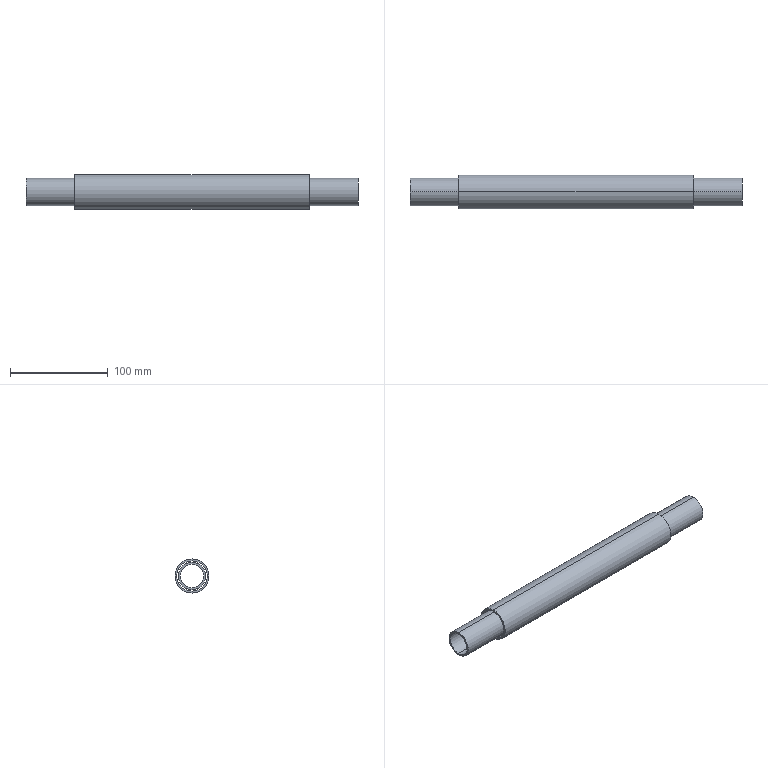Part | STEP file | VIB-C1-1-8-vibration damping pipe 28_default_machined_ | 2 solids | 12 faces | box 340 x 35 x 35 mm | volume 105306 mm3 | cylinder 8 | plane 4 | commonest cylinder face diameters 24 x2 28 x2 31 x2 35 x2
STEP:
#1=CARTESIAN_POINT('',(0.,0.,0.));
#2=DIRECTION('',(0.,0.,1.));
#3=DIRECTION('',(1.,0.,0.));
#4=AXIS2_PLACEMENT_3D('',#1,#2,#3);
#5=CARTESIAN_POINT('',(340.,0.,14.));
#6=VERTEX_POINT('',#5);
#7=CARTESIAN_POINT('',(340.,0.,-14.));
#8=VERTEX_POINT('',#7);
#9=CARTESIAN_POINT('',(340.,0.,0.));
#10=DIRECTION('',(-1.,0.,0.));
#11=DIRECTION('',(0.,0.,1.));
#12=AXIS2_PLACEMENT_3D('',#9,#10,#11);
#13=CIRCLE('',#12,14.);
#14=CARTESIAN_POINT('',(340.,0.,0.));
#15=DIRECTION('',(-1.,0.,0.));
#16=DIRECTION('',(0.,0.,1.));
#17=AXIS2_PLACEMENT_3D('',#14,#15,#16);
#18=CYLINDRICAL_SURFACE('',#17,14.);
#19=CARTESIAN_POINT('',(0.,0.));
#20=DIRECTION('',(1.,0.));
#21=VECTOR('',#20,1.);
#22=LINE('',#19,#21);
#23=(GEOMETRIC_REPRESENTATION_CONTEXT(2)PARAMETRIC_REPRESENTATION_CONTEXT()REPRESENTATION_CONTEXT('',''));
#24=DEFINITIONAL_REPRESENTATION('',(#22),#23);
#25=PCURVE('',#18,#24);
#26=CARTESIAN_POINT('',(340.,0.,0.));
#27=DIRECTION('',(1.,0.,0.));
#28=DIRECTION('',(0.,0.,-1.));
#29=AXIS2_PLACEMENT_3D('',#26,#27,#28);
#30=PLANE('',#29);
#31=CARTESIAN_POINT('',(-14.,0.));
#32=CARTESIAN_POINT('',(-14.,24.249));
#33=CARTESIAN_POINT('',(7.,12.124));
#34=CARTESIAN_POINT('',(28.,0.));
#35=CARTESIAN_POINT('',(7.,-12.124));
#36=CARTESIAN_POINT('',(-14.,-24.249));
#37=CARTESIAN_POINT('',(-14.,0.));
#38=(BOUNDED_CURVE()B_SPLINE_CURVE(2,(#31,#32,#33,#34,#35,#36,#37),.UNSPECIFIED.,.T.,.F.)B_SPLINE_CURVE_WITH_KNOTS((1,2,2,2,2,1),(-2.094,0.,2.094,4.189,6.283,8.378),.UNSPECIFIED.)CURVE()GEOMETRIC_REPRESENTATION_ITEM()RATIONAL_B_SPLINE_CURVE((1.,0.5,1.,0.5,1.,0.5,1.))REPRESENTATION_ITEM(''));
#39=(GEOMETRIC_REPRESENTATION_CONTEXT(2)PARAMETRIC_REPRESENTATION_CONTEXT()REPRESENTATION_CONTEXT('',''));
#40=DEFINITIONAL_REPRESENTATION('',(#38),#39);
#41=PCURVE('',#30,#40);
#42=SURFACE_CURVE('',#13,(#25,#41),.PCURVE_S1.);
#43=EDGE_CURVE('',#6,#8,#42,.T.);
#44=ORIENTED_EDGE('',*,*,#43,.T.);
#45=CARTESIAN_POINT('',(0.,0.,-14.));
#46=VERTEX_POINT('',#45);
#47=CARTESIAN_POINT('',(340.,0.,-14.));
#48=DIRECTION('',(-1.,0.,0.));
#49=VECTOR('',#48,1.);
#50=LINE('',#47,#49);
#51=CARTESIAN_POINT('',(3.142,0.));
#52=DIRECTION('',(0.,1.));
#53=VECTOR('',#52,1.);
#54=LINE('',#51,#53);
#55=(GEOMETRIC_REPRESENTATION_CONTEXT(2)PARAMETRIC_REPRESENTATION_CONTEXT()REPRESENTATION_CONTEXT('',''));
#56=DEFINITIONAL_REPRESENTATION('',(#54),#55);
#57=PCURVE('',#18,#56);
#58=CARTESIAN_POINT('',(340.,0.,0.));
#59=DIRECTION('',(-1.,0.,0.));
#60=DIRECTION('',(0.,0.,1.));
#61=AXIS2_PLACEMENT_3D('',#58,#59,#60);
#62=CYLINDRICAL_SURFACE('',#61,14.);
#63=CARTESIAN_POINT('',(3.142,0.));
#64=DIRECTION('',(0.,1.));
#65=VECTOR('',#64,1.);
#66=LINE('',#63,#65);
#67=(GEOMETRIC_REPRESENTATION_CONTEXT(2)PARAMETRIC_REPRESENTATION_CONTEXT()REPRESENTATION_CONTEXT('',''));
#68=DEFINITIONAL_REPRESENTATION('',(#66),#67);
#69=PCURVE('',#62,#68);
#70=SURFACE_CURVE('',#50,(#57,#69),.PCURVE_S1.);
#71=EDGE_CURVE('',#8,#46,#70,.T.);
#72=ORIENTED_EDGE('',*,*,#71,.T.);
#73=CARTESIAN_POINT('',(0.,0.,14.));
#74=VERTEX_POINT('',#73);
#75=CARTESIAN_POINT('',(0.,0.,0.));
#76=DIRECTION('',(1.,0.,0.));
#77=DIRECTION('',(0.,0.,1.));
#78=AXIS2_PLACEMENT_3D('',#75,#76,#77);
#79=CIRCLE('',#78,14.);
#80=CARTESIAN_POINT('',(6.283,340.));
#81=DIRECTION('',(-1.,0.));
#82=VECTOR('',#81,1.);
#83=LINE('',#80,#82);
#84=(GEOMETRIC_REPRESENTATION_CONTEXT(2)PARAMETRIC_REPRESENTATION_CONTEXT()REPRESENTATION_CONTEXT('',''));
#85=DEFINITIONAL_REPRESENTATION('',(#83),#84);
#86=PCURVE('',#18,#85);
#87=CARTESIAN_POINT('',(0.,0.,0.));
#88=DIRECTION('',(1.,0.,0.));
#89=DIRECTION('',(0.,0.,-1.));
#90=AXIS2_PLACEMENT_3D('',#87,#88,#89);
#91=PLANE('',#90);
#92=CARTESIAN_POINT('',(0.,0.));
#93=DIRECTION('',(-1.,0.));
#94=AXIS2_PLACEMENT_2D('',#92,#93);
#95=CIRCLE('',#94,14.);
#96=(GEOMETRIC_REPRESENTATION_CONTEXT(2)PARAMETRIC_REPRESENTATION_CONTEXT()REPRESENTATION_CONTEXT('',''));
#97=DEFINITIONAL_REPRESENTATION('',(#95),#96);
#98=PCURVE('',#91,#97);
#99=SURFACE_CURVE('',#79,(#86,#98),.PCURVE_S1.);
#100=EDGE_CURVE('',#46,#74,#99,.T.);
#101=ORIENTED_EDGE('',*,*,#100,.T.);
#102=CARTESIAN_POINT('',(340.,0.,14.));
#103=DIRECTION('',(-1.,0.,0.));
#104=VECTOR('',#103,1.);
#105=LINE('',#102,#104);
#106=CARTESIAN_POINT('',(0.,0.));
#107=DIRECTION('',(0.,1.));
#108=VECTOR('',#107,1.);
#109=LINE('',#106,#108);
#110=(GEOMETRIC_REPRESENTATION_CONTEXT(2)PARAMETRIC_REPRESENTATION_CONTEXT()REPRESENTATION_CONTEXT('',''));
#111=DEFINITIONAL_REPRESENTATION('',(#109),#110);
#112=PCURVE('',#18,#111);
#113=CARTESIAN_POINT('',(6.283,0.));
#114=DIRECTION('',(0.,1.));
#115=VECTOR('',#114,1.);
#116=LINE('',#113,#115);
#117=(GEOMETRIC_REPRESENTATION_CONTEXT(2)PARAMETRIC_REPRESENTATION_CONTEXT()REPRESENTATION_CONTEXT('',''));
#118=DEFINITIONAL_REPRESENTATION('',(#116),#117);
#119=PCURVE('',#62,#118);
#120=SURFACE_CURVE('',#105,(#112,#119),.PCURVE_S1.);
#121=EDGE_CURVE('',#6,#74,#120,.T.);
#122=ORIENTED_EDGE('',*,*,#121,.F.);
#123=EDGE_LOOP('',(#44,#72,#101,#122));
#124=FACE_BOUND('',#123,.T.);
#125=ADVANCED_FACE('',(#124),#18,.T.);
#126=CARTESIAN_POINT('',(340.,0.,12.));
#127=VERTEX_POINT('',#126);
#128=CARTESIAN_POINT('',(0.,0.,12.));
#129=VERTEX_POINT('',#128);
#130=CARTESIAN_POINT('',(340.,0.,12.));
#131=DIRECTION('',(-1.,0.,0.));
#132=VECTOR('',#131,1.);
#133=LINE('',#130,#132);
#134=CARTESIAN_POINT('',(340.,0.,0.));
#135=DIRECTION('',(-1.,0.,0.));
#136=DIRECTION('',(0.,0.,1.));
#137=AXIS2_PLACEMENT_3D('',#134,#135,#136);
#138=CYLINDRICAL_SURFACE('',#137,12.);
#139=CARTESIAN_POINT('',(6.283,0.));
#140=DIRECTION('',(0.,1.));
#141=VECTOR('',#140,1.);
#142=LINE('',#139,#141);
#143=(GEOMETRIC_REPRESENTATION_CONTEXT(2)PARAMETRIC_REPRESENTATION_CONTEXT()REPRESENTATION_CONTEXT('',''));
#144=DEFINITIONAL_REPRESENTATION('',(#142),#143);
#145=PCURVE('',#138,#144);
#146=CARTESIAN_POINT('',(340.,0.,0.));
#147=DIRECTION('',(-1.,0.,0.));
#148=DIRECTION('',(0.,0.,1.));
#149=AXIS2_PLACEMENT_3D('',#146,#147,#148);
#150=CYLINDRICAL_SURFACE('',#149,12.);
#151=CARTESIAN_POINT('',(0.,0.));
#152=DIRECTION('',(0.,1.));
#153=VECTOR('',#152,1.);
#154=LINE('',#151,#153);
#155=(GEOMETRIC_REPRESENTATION_CONTEXT(2)PARAMETRIC_REPRESENTATION_CONTEXT()REPRESENTATION_CONTEXT('',''));
#156=DEFINITIONAL_REPRESENTATION('',(#154),#155);
#157=PCURVE('',#150,#156);
#158=SURFACE_CURVE('',#133,(#145,#157),.PCURVE_S1.);
#159=EDGE_CURVE('',#127,#129,#158,.T.);
#160=ORIENTED_EDGE('',*,*,#159,.T.);
#161=CARTESIAN_POINT('',(0.,0.,-12.));
#162=VERTEX_POINT('',#161);
#163=CARTESIAN_POINT('',(0.,0.,0.));
#164=DIRECTION('',(-1.,0.,0.));
#165=DIRECTION('',(0.,0.,1.));
#166=AXIS2_PLACEMENT_3D('',#163,#164,#165);
#167=CIRCLE('',#166,12.);
#168=CARTESIAN_POINT('',(0.,340.));
#169=DIRECTION('',(1.,0.));
#170=VECTOR('',#169,1.);
#171=LINE('',#168,#170);
#172=(GEOMETRIC_REPRESENTATION_CONTEXT(2)PARAMETRIC_REPRESENTATION_CONTEXT()REPRESENTATION_CONTEXT('',''));
#173=DEFINITIONAL_REPRESENTATION('',(#171),#172);
#174=PCURVE('',#138,#173);
#175=CARTESIAN_POINT('',(-12.,0.));
#176=CARTESIAN_POINT('',(-12.,20.785));
#177=CARTESIAN_POINT('',(6.,10.392));
#178=CARTESIAN_POINT('',(24.,0.));
#179=CARTESIAN_POINT('',(6.,-10.392));
#180=CARTESIAN_POINT('',(-12.,-20.785));
#181=CARTESIAN_POINT('',(-12.,0.));
#182=(BOUNDED_CURVE()B_SPLINE_CURVE(2,(#175,#176,#177,#178,#179,#180,#181),.UNSPECIFIED.,.T.,.F.)B_SPLINE_CURVE_WITH_KNOTS((1,2,2,2,2,1),(-2.094,0.,2.094,4.189,6.283,8.378),.UNSPECIFIED.)CURVE()GEOMETRIC_REPRESENTATION_ITEM()RATIONAL_B_SPLINE_CURVE((1.,0.5,1.,0.5,1.,0.5,1.))REPRESENTATION_ITEM(''));
#183=(GEOMETRIC_REPRESENTATION_CONTEXT(2)PARAMETRIC_REPRESENTATION_CONTEXT()REPRESENTATION_CONTEXT('',''));
#184=DEFINITIONAL_REPRESENTATION('',(#182),#183);
#185=PCURVE('',#91,#184);
#186=SURFACE_CURVE('',#167,(#174,#185),.PCURVE_S1.);
#187=EDGE_CURVE('',#162,#129,#186,.T.);
#188=ORIENTED_EDGE('',*,*,#187,.F.);
#189=CARTESIAN_POINT('',(340.,0.,-12.));
#190=VERTEX_POINT('',#189);
#191=CARTESIAN_POINT('',(340.,0.,-12.));
#192=DIRECTION('',(-1.,0.,0.));
#193=VECTOR('',#192,1.);
#194=LINE('',#191,#193);
#195=CARTESIAN_POINT('',(3.142,0.));
#196=DIRECTION('',(0.,1.));
#197=VECTOR('',#196,1.);
#198=LINE('',#195,#197);
#199=(GEOMETRIC_REPRESENTATION_CONTEXT(2)PARAMETRIC_REPRESENTATION_CONTEXT()REPRESENTATION_CONTEXT('',''));
#200=DEFINITIONAL_REPRESENTATION('',(#198),#199);
#201=PCURVE('',#138,#200);
#202=CARTESIAN_POINT('',(3.142,0.));
#203=DIRECTION('',(0.,1.));
#204=VECTOR('',#203,1.);
#205=LINE('',#202,#204);
#206=(GEOMETRIC_REPRESENTATION_CONTEXT(2)PARAMETRIC_REPRESENTATION_CONTEXT()REPRESENTATION_CONTEXT('',''));
#207=DEFINITIONAL_REPRESENTATION('',(#205),#206);
#208=PCURVE('',#150,#207);
#209=SURFACE_CURVE('',#194,(#201,#208),.PCURVE_S1.);
#210=EDGE_CURVE('',#190,#162,#209,.T.);
#211=ORIENTED_EDGE('',*,*,#210,.F.);
#212=CARTESIAN_POINT('',(340.,0.,0.));
#213=DIRECTION('',(-1.,0.,0.));
#214=DIRECTION('',(0.,0.,1.));
#215=AXIS2_PLACEMENT_3D('',#212,#213,#214);
#216=CIRCLE('',#215,12.);
#217=CARTESIAN_POINT('',(0.,0.));
#218=DIRECTION('',(1.,0.));
#219=VECTOR('',#218,1.);
#220=LINE('',#217,#219);
#221=(GEOMETRIC_REPRESENTATION_CONTEXT(2)PARAMETRIC_REPRESENTATION_CONTEXT()REPRESENTATION_CONTEXT('',''));
#222=DEFINITIONAL_REPRESENTATION('',(#220),#221);
#223=PCURVE('',#138,#222);
#224=CARTESIAN_POINT('',(-12.,0.));
#225=CARTESIAN_POINT('',(-12.,20.785));
#226=CARTESIAN_POINT('',(6.,10.392));
#227=CARTESIAN_POINT('',(24.,0.));
#228=CARTESIAN_POINT('',(6.,-10.392));
#229=CARTESIAN_POINT('',(-12.,-20.785));
#230=CARTESIAN_POINT('',(-12.,0.));
#231=(BOUNDED_CURVE()B_SPLINE_CURVE(2,(#224,#225,#226,#227,#228,#229,#230),.UNSPECIFIED.,.T.,.F.)B_SPLINE_CURVE_WITH_KNOTS((1,2,2,2,2,1),(-2.094,0.,2.094,4.189,6.283,8.378),.UNSPECIFIED.)CURVE()GEOMETRIC_REPRESENTATION_ITEM()RATIONAL_B_SPLINE_CURVE((1.,0.5,1.,0.5,1.,0.5,1.))REPRESENTATION_ITEM(''));
#232=(GEOMETRIC_REPRESENTATION_CONTEXT(2)PARAMETRIC_REPRESENTATION_CONTEXT()REPRESENTATION_CONTEXT('',''));
#233=DEFINITIONAL_REPRESENTATION('',(#231),#232);
#234=PCURVE('',#30,#233);
#235=SURFACE_CURVE('',#216,(#223,#234),.PCURVE_S1.);
#236=EDGE_CURVE('',#190,#127,#235,.T.);
#237=ORIENTED_EDGE('',*,*,#236,.T.);
#238=EDGE_LOOP('',(#160,#188,#211,#237));
#239=FACE_BOUND('',#238,.F.);
#240=ADVANCED_FACE('',(#239),#138,.F.);
#241=ORIENTED_EDGE('',*,*,#71,.F.);
#242=CARTESIAN_POINT('',(340.,0.,0.));
#243=DIRECTION('',(-1.,0.,0.));
#244=DIRECTION('',(0.,0.,1.));
#245=AXIS2_PLACEMENT_3D('',#242,#243,#244);
#246=CIRCLE('',#245,14.);
#247=CARTESIAN_POINT('',(0.,0.));
#248=DIRECTION('',(1.,0.));
#249=VECTOR('',#248,1.);
#250=LINE('',#247,#249);
#251=(GEOMETRIC_REPRESENTATION_CONTEXT(2)PARAMETRIC_REPRESENTATION_CONTEXT()REPRESENTATION_CONTEXT('',''));
#252=DEFINITIONAL_REPRESENTATION('',(#250),#251);
#253=PCURVE('',#62,#252);
#254=CARTESIAN_POINT('',(-14.,0.));
#255=CARTESIAN_POINT('',(-14.,24.249));
#256=CARTESIAN_POINT('',(7.,12.124));
#257=CARTESIAN_POINT('',(28.,0.));
#258=CARTESIAN_POINT('',(7.,-12.124));
#259=CARTESIAN_POINT('',(-14.,-24.249));
#260=CARTESIAN_POINT('',(-14.,0.));
#261=(BOUNDED_CURVE()B_SPLINE_CURVE(2,(#254,#255,#256,#257,#258,#259,#260),.UNSPECIFIED.,.T.,.F.)B_SPLINE_CURVE_WITH_KNOTS((1,2,2,2,2,1),(-2.094,0.,2.094,4.189,6.283,8.378),.UNSPECIFIED.)CURVE()GEOMETRIC_REPRESENTATION_ITEM()RATIONAL_B_SPLINE_CURVE((1.,0.5,1.,0.5,1.,0.5,1.))REPRESENTATION_ITEM(''));
#262=(GEOMETRIC_REPRESENTATION_CONTEXT(2)PARAMETRIC_REPRESENTATION_CONTEXT()REPRESENTATION_CONTEXT('',''));
#263=DEFINITIONAL_REPRESENTATION('',(#261),#262);
#264=PCURVE('',#30,#263);
#265=SURFACE_CURVE('',#246,(#253,#264),.PCURVE_S1.);
#266=EDGE_CURVE('',#8,#6,#265,.T.);
#267=ORIENTED_EDGE('',*,*,#266,.T.);
#268=ORIENTED_EDGE('',*,*,#121,.T.);
#269=CARTESIAN_POINT('',(0.,0.,0.));
#270=DIRECTION('',(1.,0.,0.));
#271=DIRECTION('',(0.,0.,1.));
#272=AXIS2_PLACEMENT_3D('',#269,#270,#271);
#273=CIRCLE('',#272,14.);
#274=CARTESIAN_POINT('',(6.283,340.));
#275=DIRECTION('',(-1.,0.));
#276=VECTOR('',#275,1.);
#277=LINE('',#274,#276);
#278=(GEOMETRIC_REPRESENTATION_CONTEXT(2)PARAMETRIC_REPRESENTATION_CONTEXT()REPRESENTATION_CONTEXT('',''));
#279=DEFINITIONAL_REPRESENTATION('',(#277),#278);
#280=PCURVE('',#62,#279);
#281=CARTESIAN_POINT('',(0.,0.));
#282=DIRECTION('',(-1.,0.));
#283=AXIS2_PLACEMENT_2D('',#281,#282);
#284=CIRCLE('',#283,14.);
#285=(GEOMETRIC_REPRESENTATION_CONTEXT(2)PARAMETRIC_REPRESENTATION_CONTEXT()REPRESENTATION_CONTEXT('',''));
#286=DEFINITIONAL_REPRESENTATION('',(#284),#285);
#287=PCURVE('',#91,#286);
#288=SURFACE_CURVE('',#273,(#280,#287),.PCURVE_S1.);
#289=EDGE_CURVE('',#74,#46,#288,.T.);
#290=ORIENTED_EDGE('',*,*,#289,.T.);
#291=EDGE_LOOP('',(#241,#267,#268,#290));
#292=FACE_BOUND('',#291,.T.);
#293=ADVANCED_FACE('',(#292),#62,.T.);
#294=ORIENTED_EDGE('',*,*,#289,.F.);
#295=ORIENTED_EDGE('',*,*,#100,.F.);
#296=EDGE_LOOP('',(#294,#295));
#297=FACE_BOUND('',#296,.T.);
#298=CARTESIAN_POINT('',(0.,0.,0.));
#299=DIRECTION('',(-1.,0.,0.));
#300=DIRECTION('',(0.,0.,1.));
#301=AXIS2_PLACEMENT_3D('',#298,#299,#300);
#302=CIRCLE('',#301,12.);
#303=CARTESIAN_POINT('',(-12.,0.));
#304=CARTESIAN_POINT('',(-12.,20.785));
#305=CARTESIAN_POINT('',(6.,10.392));
#306=CARTESIAN_POINT('',(24.,0.));
#307=CARTESIAN_POINT('',(6.,-10.392));
#308=CARTESIAN_POINT('',(-12.,-20.785));
#309=CARTESIAN_POINT('',(-12.,0.));
#310=(BOUNDED_CURVE()B_SPLINE_CURVE(2,(#303,#304,#305,#306,#307,#308,#309),.UNSPECIFIED.,.T.,.F.)B_SPLINE_CURVE_WITH_KNOTS((1,2,2,2,2,1),(-2.094,0.,2.094,4.189,6.283,8.378),.UNSPECIFIED.)CURVE()GEOMETRIC_REPRESENTATION_ITEM()RATIONAL_B_SPLINE_CURVE((1.,0.5,1.,0.5,1.,0.5,1.))REPRESENTATION_ITEM(''));
#311=(GEOMETRIC_REPRESENTATION_CONTEXT(2)PARAMETRIC_REPRESENTATION_CONTEXT()REPRESENTATION_CONTEXT('',''));
#312=DEFINITIONAL_REPRESENTATION('',(#310),#311);
#313=PCURVE('',#91,#312);
#314=CARTESIAN_POINT('',(0.,340.));
#315=DIRECTION('',(1.,0.));
#316=VECTOR('',#315,1.);
#317=LINE('',#314,#316);
#318=(GEOMETRIC_REPRESENTATION_CONTEXT(2)PARAMETRIC_REPRESENTATION_CONTEXT()REPRESENTATION_CONTEXT('',''));
#319=DEFINITIONAL_REPRESENTATION('',(#317),#318);
#320=PCURVE('',#150,#319);
#321=SURFACE_CURVE('',#302,(#313,#320),.PCURVE_S1.);
#322=EDGE_CURVE('',#129,#162,#321,.T.);
#323=ORIENTED_EDGE('',*,*,#322,.F.);
#324=ORIENTED_EDGE('',*,*,#187,.F.);
#325=EDGE_LOOP('',(#323,#324));
#326=FACE_BOUND('',#325,.T.);
#327=ADVANCED_FACE('',(#297,#326),#91,.F.);
#328=ORIENTED_EDGE('',*,*,#43,.F.);
#329=ORIENTED_EDGE('',*,*,#266,.F.);
#330=EDGE_LOOP('',(#328,#329));
#331=FACE_BOUND('',#330,.T.);
#332=CARTESIAN_POINT('',(340.,0.,0.));
#333=DIRECTION('',(-1.,0.,0.));
#334=DIRECTION('',(0.,0.,1.));
#335=AXIS2_PLACEMENT_3D('',#332,#333,#334);
#336=CIRCLE('',#335,12.);
#337=CARTESIAN_POINT('',(-12.,0.));
#338=CARTESIAN_POINT('',(-12.,20.785));
#339=CARTESIAN_POINT('',(6.,10.392));
#340=CARTESIAN_POINT('',(24.,0.));
#341=CARTESIAN_POINT('',(6.,-10.392));
#342=CARTESIAN_POINT('',(-12.,-20.785));
#343=CARTESIAN_POINT('',(-12.,0.));
#344=(BOUNDED_CURVE()B_SPLINE_CURVE(2,(#337,#338,#339,#340,#341,#342,#343),.UNSPECIFIED.,.T.,.F.)B_SPLINE_CURVE_WITH_KNOTS((1,2,2,2,2,1),(-2.094,0.,2.094,4.189,6.283,8.378),.UNSPECIFIED.)CURVE()GEOMETRIC_REPRESENTATION_ITEM()RATIONAL_B_SPLINE_CURVE((1.,0.5,1.,0.5,1.,0.5,1.))REPRESENTATION_ITEM(''));
#345=(GEOMETRIC_REPRESENTATION_CONTEXT(2)PARAMETRIC_REPRESENTATION_CONTEXT()REPRESENTATION_CONTEXT('',''));
#346=DEFINITIONAL_REPRESENTATION('',(#344),#345);
#347=PCURVE('',#30,#346);
#348=CARTESIAN_POINT('',(0.,0.));
#349=DIRECTION('',(1.,0.));
#350=VECTOR('',#349,1.);
#351=LINE('',#348,#350);
#352=(GEOMETRIC_REPRESENTATION_CONTEXT(2)PARAMETRIC_REPRESENTATION_CONTEXT()REPRESENTATION_CONTEXT('',''));
#353=DEFINITIONAL_REPRESENTATION('',(#351),#352);
#354=PCURVE('',#150,#353);
#355=SURFACE_CURVE('',#336,(#347,#354),.PCURVE_S1.);
#356=EDGE_CURVE('',#127,#190,#355,.T.);
#357=ORIENTED_EDGE('',*,*,#356,.T.);
#358=ORIENTED_EDGE('',*,*,#236,.T.);
#359=EDGE_LOOP('',(#357,#358));
#360=FACE_BOUND('',#359,.T.);
#361=ADVANCED_FACE('',(#331,#360),#30,.T.);
#362=ORIENTED_EDGE('',*,*,#322,.F.);
#363=ORIENTED_EDGE('',*,*,#159,.F.);
#364=ORIENTED_EDGE('',*,*,#356,.T.);
#365=ORIENTED_EDGE('',*,*,#210,.T.);
#366=EDGE_LOOP('',(#362,#363,#364,#365));
#367=FACE_BOUND('',#366,.F.);
#368=ADVANCED_FACE('',(#367),#150,.F.);
#369=CLOSED_SHELL('',(#125,#240,#293,#327,#361,#368));
#370=MANIFOLD_SOLID_BREP('',#369);
#371=CARTESIAN_POINT('',(290.,0.,17.5));
#372=VERTEX_POINT('',#371);
#373=CARTESIAN_POINT('',(290.,0.,-17.5));
#374=VERTEX_POINT('',#373);
#375=CARTESIAN_POINT('',(290.,0.,0.));
#376=DIRECTION('',(-1.,0.,0.));
#377=DIRECTION('',(0.,0.,1.));
#378=AXIS2_PLACEMENT_3D('',#375,#376,#377);
#379=CIRCLE('',#378,17.5);
#380=CARTESIAN_POINT('',(290.,0.,0.));
#381=DIRECTION('',(-1.,0.,0.));
#382=DIRECTION('',(0.,0.,1.));
#383=AXIS2_PLACEMENT_3D('',#380,#381,#382);
#384=CYLINDRICAL_SURFACE('',#383,17.5);
#385=CARTESIAN_POINT('',(0.,0.));
#386=DIRECTION('',(1.,0.));
#387=VECTOR('',#386,1.);
#388=LINE('',#385,#387);
#389=(GEOMETRIC_REPRESENTATION_CONTEXT(2)PARAMETRIC_REPRESENTATION_CONTEXT()REPRESENTATION_CONTEXT('',''));
#390=DEFINITIONAL_REPRESENTATION('',(#388),#389);
#391=PCURVE('',#384,#390);
#392=CARTESIAN_POINT('',(290.,0.,0.));
#393=DIRECTION('',(1.,0.,0.));
#394=DIRECTION('',(0.,0.,-1.));
#395=AXIS2_PLACEMENT_3D('',#392,#393,#394);
#396=PLANE('',#395);
#397=CARTESIAN_POINT('',(-17.5,0.));
#398=CARTESIAN_POINT('',(-17.5,30.311));
#399=CARTESIAN_POINT('',(8.75,15.155));
#400=CARTESIAN_POINT('',(35.,0.));
#401=CARTESIAN_POINT('',(8.75,-15.155));
#402=CARTESIAN_POINT('',(-17.5,-30.311));
#403=CARTESIAN_POINT('',(-17.5,0.));
#404=(BOUNDED_CURVE()B_SPLINE_CURVE(2,(#397,#398,#399,#400,#401,#402,#403),.UNSPECIFIED.,.T.,.F.)B_SPLINE_CURVE_WITH_KNOTS((1,2,2,2,2,1),(-2.094,0.,2.094,4.189,6.283,8.378),.UNSPECIFIED.)CURVE()GEOMETRIC_REPRESENTATION_ITEM()RATIONAL_B_SPLINE_CURVE((1.,0.5,1.,0.5,1.,0.5,1.))REPRESENTATION_ITEM(''));
#405=(GEOMETRIC_REPRESENTATION_CONTEXT(2)PARAMETRIC_REPRESENTATION_CONTEXT()REPRESENTATION_CONTEXT('',''));
#406=DEFINITIONAL_REPRESENTATION('',(#404),#405);
#407=PCURVE('',#396,#406);
#408=SURFACE_CURVE('',#379,(#391,#407),.PCURVE_S1.);
#409=EDGE_CURVE('',#372,#374,#408,.T.);
#410=ORIENTED_EDGE('',*,*,#409,.T.);
#411=CARTESIAN_POINT('',(50.,0.,-17.5));
#412=VERTEX_POINT('',#411);
#413=CARTESIAN_POINT('',(290.,0.,-17.5));
#414=DIRECTION('',(-1.,0.,0.));
#415=VECTOR('',#414,1.);
#416=LINE('',#413,#415);
#417=CARTESIAN_POINT('',(3.142,0.));
#418=DIRECTION('',(0.,1.));
#419=VECTOR('',#418,1.);
#420=LINE('',#417,#419);
#421=(GEOMETRIC_REPRESENTATION_CONTEXT(2)PARAMETRIC_REPRESENTATION_CONTEXT()REPRESENTATION_CONTEXT('',''));
#422=DEFINITIONAL_REPRESENTATION('',(#420),#421);
#423=PCURVE('',#384,#422);
#424=CARTESIAN_POINT('',(290.,0.,0.));
#425=DIRECTION('',(-1.,0.,0.));
#426=DIRECTION('',(0.,0.,1.));
#427=AXIS2_PLACEMENT_3D('',#424,#425,#426);
#428=CYLINDRICAL_SURFACE('',#427,17.5);
#429=CARTESIAN_POINT('',(3.142,0.));
#430=DIRECTION('',(0.,1.));
#431=VECTOR('',#430,1.);
#432=LINE('',#429,#431);
#433=(GEOMETRIC_REPRESENTATION_CONTEXT(2)PARAMETRIC_REPRESENTATION_CONTEXT()REPRESENTATION_CONTEXT('',''));
#434=DEFINITIONAL_REPRESENTATION('',(#432),#433);
#435=PCURVE('',#428,#434);
#436=SURFACE_CURVE('',#416,(#423,#435),.PCURVE_S1.);
#437=EDGE_CURVE('',#374,#412,#436,.T.);
#438=ORIENTED_EDGE('',*,*,#437,.T.);
#439=CARTESIAN_POINT('',(50.,0.,17.5));
#440=VERTEX_POINT('',#439);
#441=CARTESIAN_POINT('',(50.,0.,0.));
#442=DIRECTION('',(1.,0.,0.));
#443=DIRECTION('',(0.,0.,1.));
#444=AXIS2_PLACEMENT_3D('',#441,#442,#443);
#445=CIRCLE('',#444,17.5);
#446=CARTESIAN_POINT('',(6.283,240.));
#447=DIRECTION('',(-1.,0.));
#448=VECTOR('',#447,1.);
#449=LINE('',#446,#448);
#450=(GEOMETRIC_REPRESENTATION_CONTEXT(2)PARAMETRIC_REPRESENTATION_CONTEXT()REPRESENTATION_CONTEXT('',''));
#451=DEFINITIONAL_REPRESENTATION('',(#449),#450);
#452=PCURVE('',#384,#451);
#453=CARTESIAN_POINT('',(50.,0.,0.));
#454=DIRECTION('',(1.,0.,0.));
#455=DIRECTION('',(0.,0.,-1.));
#456=AXIS2_PLACEMENT_3D('',#453,#454,#455);
#457=PLANE('',#456);
#458=CARTESIAN_POINT('',(0.,0.));
#459=DIRECTION('',(-1.,0.));
#460=AXIS2_PLACEMENT_2D('',#458,#459);
#461=CIRCLE('',#460,17.5);
#462=(GEOMETRIC_REPRESENTATION_CONTEXT(2)PARAMETRIC_REPRESENTATION_CONTEXT()REPRESENTATION_CONTEXT('',''));
#463=DEFINITIONAL_REPRESENTATION('',(#461),#462);
#464=PCURVE('',#457,#463);
#465=SURFACE_CURVE('',#445,(#452,#464),.PCURVE_S1.);
#466=EDGE_CURVE('',#412,#440,#465,.T.);
#467=ORIENTED_EDGE('',*,*,#466,.T.);
#468=CARTESIAN_POINT('',(290.,0.,17.5));
#469=DIRECTION('',(-1.,0.,0.));
#470=VECTOR('',#469,1.);
#471=LINE('',#468,#470);
#472=CARTESIAN_POINT('',(0.,0.));
#473=DIRECTION('',(0.,1.));
#474=VECTOR('',#473,1.);
#475=LINE('',#472,#474);
#476=(GEOMETRIC_REPRESENTATION_CONTEXT(2)PARAMETRIC_REPRESENTATION_CONTEXT()REPRESENTATION_CONTEXT('',''));
#477=DEFINITIONAL_REPRESENTATION('',(#475),#476);
#478=PCURVE('',#384,#477);
#479=CARTESIAN_POINT('',(6.283,0.));
#480=DIRECTION('',(0.,1.));
#481=VECTOR('',#480,1.);
#482=LINE('',#479,#481);
#483=(GEOMETRIC_REPRESENTATION_CONTEXT(2)PARAMETRIC_REPRESENTATION_CONTEXT()REPRESENTATION_CONTEXT('',''));
#484=DEFINITIONAL_REPRESENTATION('',(#482),#483);
#485=PCURVE('',#428,#484);
#486=SURFACE_CURVE('',#471,(#478,#485),.PCURVE_S1.);
#487=EDGE_CURVE('',#372,#440,#486,.T.);
#488=ORIENTED_EDGE('',*,*,#487,.F.);
#489=EDGE_LOOP('',(#410,#438,#467,#488));
#490=FACE_BOUND('',#489,.T.);
#491=ADVANCED_FACE('',(#490),#384,.T.);
#492=CARTESIAN_POINT('',(290.,0.,15.5));
#493=VERTEX_POINT('',#492);
#494=CARTESIAN_POINT('',(50.,0.,15.5));
#495=VERTEX_POINT('',#494);
#496=CARTESIAN_POINT('',(290.,0.,15.5));
#497=DIRECTION('',(-1.,0.,0.));
#498=VECTOR('',#497,1.);
#499=LINE('',#496,#498);
#500=CARTESIAN_POINT('',(290.,0.,0.));
#501=DIRECTION('',(-1.,0.,0.));
#502=DIRECTION('',(0.,0.,1.));
#503=AXIS2_PLACEMENT_3D('',#500,#501,#502);
#504=CYLINDRICAL_SURFACE('',#503,15.5);
#505=CARTESIAN_POINT('',(6.283,0.));
#506=DIRECTION('',(0.,1.));
#507=VECTOR('',#506,1.);
#508=LINE('',#505,#507);
#509=(GEOMETRIC_REPRESENTATION_CONTEXT(2)PARAMETRIC_REPRESENTATION_CONTEXT()REPRESENTATION_CONTEXT('',''));
#510=DEFINITIONAL_REPRESENTATION('',(#508),#509);
#511=PCURVE('',#504,#510);
#512=CARTESIAN_POINT('',(290.,0.,0.));
#513=DIRECTION('',(-1.,0.,0.));
#514=DIRECTION('',(0.,0.,1.));
#515=AXIS2_PLACEMENT_3D('',#512,#513,#514);
#516=CYLINDRICAL_SURFACE('',#515,15.5);
#517=CARTESIAN_POINT('',(0.,0.));
#518=DIRECTION('',(0.,1.));
#519=VECTOR('',#518,1.);
#520=LINE('',#517,#519);
#521=(GEOMETRIC_REPRESENTATION_CONTEXT(2)PARAMETRIC_REPRESENTATION_CONTEXT()REPRESENTATION_CONTEXT('',''));
#522=DEFINITIONAL_REPRESENTATION('',(#520),#521);
#523=PCURVE('',#516,#522);
#524=SURFACE_CURVE('',#499,(#511,#523),.PCURVE_S1.);
#525=EDGE_CURVE('',#493,#495,#524,.T.);
#526=ORIENTED_EDGE('',*,*,#525,.T.);
#527=CARTESIAN_POINT('',(50.,0.,-15.5));
#528=VERTEX_POINT('',#527);
#529=CARTESIAN_POINT('',(50.,0.,0.));
#530=DIRECTION('',(-1.,0.,0.));
#531=DIRECTION('',(0.,0.,1.));
#532=AXIS2_PLACEMENT_3D('',#529,#530,#531);
#533=CIRCLE('',#532,15.5);
#534=CARTESIAN_POINT('',(0.,240.));
#535=DIRECTION('',(1.,0.));
#536=VECTOR('',#535,1.);
#537=LINE('',#534,#536);
#538=(GEOMETRIC_REPRESENTATION_CONTEXT(2)PARAMETRIC_REPRESENTATION_CONTEXT()REPRESENTATION_CONTEXT('',''));
#539=DEFINITIONAL_REPRESENTATION('',(#537),#538);
#540=PCURVE('',#504,#539);
#541=CARTESIAN_POINT('',(-15.5,0.));
#542=CARTESIAN_POINT('',(-15.5,26.847));
#543=CARTESIAN_POINT('',(7.75,13.423));
#544=CARTESIAN_POINT('',(31.,0.));
#545=CARTESIAN_POINT('',(7.75,-13.423));
#546=CARTESIAN_POINT('',(-15.5,-26.847));
#547=CARTESIAN_POINT('',(-15.5,0.));
#548=(BOUNDED_CURVE()B_SPLINE_CURVE(2,(#541,#542,#543,#544,#545,#546,#547),.UNSPECIFIED.,.T.,.F.)B_SPLINE_CURVE_WITH_KNOTS((1,2,2,2,2,1),(-2.094,0.,2.094,4.189,6.283,8.378),.UNSPECIFIED.)CURVE()GEOMETRIC_REPRESENTATION_ITEM()RATIONAL_B_SPLINE_CURVE((1.,0.5,1.,0.5,1.,0.5,1.))REPRESENTATION_ITEM(''));
#549=(GEOMETRIC_REPRESENTATION_CONTEXT(2)PARAMETRIC_REPRESENTATION_CONTEXT()REPRESENTATION_CONTEXT('',''));
#550=DEFINITIONAL_REPRESENTATION('',(#548),#549);
#551=PCURVE('',#457,#550);
#552=SURFACE_CURVE('',#533,(#540,#551),.PCURVE_S1.);
#553=EDGE_CURVE('',#528,#495,#552,.T.);
#554=ORIENTED_EDGE('',*,*,#553,.F.);
#555=CARTESIAN_POINT('',(290.,0.,-15.5));
#556=VERTEX_POINT('',#555);
#557=CARTESIAN_POINT('',(290.,0.,-15.5));
#558=DIRECTION('',(-1.,0.,0.));
#559=VECTOR('',#558,1.);
#560=LINE('',#557,#559);
#561=CARTESIAN_POINT('',(3.142,0.));
#562=DIRECTION('',(0.,1.));
#563=VECTOR('',#562,1.);
#564=LINE('',#561,#563);
#565=(GEOMETRIC_REPRESENTATION_CONTEXT(2)PARAMETRIC_REPRESENTATION_CONTEXT()REPRESENTATION_CONTEXT('',''));
#566=DEFINITIONAL_REPRESENTATION('',(#564),#565);
#567=PCURVE('',#504,#566);
#568=CARTESIAN_POINT('',(3.142,0.));
#569=DIRECTION('',(0.,1.));
#570=VECTOR('',#569,1.);
#571=LINE('',#568,#570);
#572=(GEOMETRIC_REPRESENTATION_CONTEXT(2)PARAMETRIC_REPRESENTATION_CONTEXT()REPRESENTATION_CONTEXT('',''));
#573=DEFINITIONAL_REPRESENTATION('',(#571),#572);
#574=PCURVE('',#516,#573);
#575=SURFACE_CURVE('',#560,(#567,#574),.PCURVE_S1.);
#576=EDGE_CURVE('',#556,#528,#575,.T.);
#577=ORIENTED_EDGE('',*,*,#576,.F.);
#578=CARTESIAN_POINT('',(290.,0.,0.));
#579=DIRECTION('',(-1.,0.,0.));
#580=DIRECTION('',(0.,0.,1.));
#581=AXIS2_PLACEMENT_3D('',#578,#579,#580);
#582=CIRCLE('',#581,15.5);
#583=CARTESIAN_POINT('',(0.,0.));
#584=DIRECTION('',(1.,0.));
#585=VECTOR('',#584,1.);
#586=LINE('',#583,#585);
#587=(GEOMETRIC_REPRESENTATION_CONTEXT(2)PARAMETRIC_REPRESENTATION_CONTEXT()REPRESENTATION_CONTEXT('',''));
#588=DEFINITIONAL_REPRESENTATION('',(#586),#587);
#589=PCURVE('',#504,#588);
#590=CARTESIAN_POINT('',(-15.5,0.));
#591=CARTESIAN_POINT('',(-15.5,26.847));
#592=CARTESIAN_POINT('',(7.75,13.423));
#593=CARTESIAN_POINT('',(31.,0.));
#594=CARTESIAN_POINT('',(7.75,-13.423));
#595=CARTESIAN_POINT('',(-15.5,-26.847));
#596=CARTESIAN_POINT('',(-15.5,0.));
#597=(BOUNDED_CURVE()B_SPLINE_CURVE(2,(#590,#591,#592,#593,#594,#595,#596),.UNSPECIFIED.,.T.,.F.)B_SPLINE_CURVE_WITH_KNOTS((1,2,2,2,2,1),(-2.094,0.,2.094,4.189,6.283,8.378),.UNSPECIFIED.)CURVE()GEOMETRIC_REPRESENTATION_ITEM()RATIONAL_B_SPLINE_CURVE((1.,0.5,1.,0.5,1.,0.5,1.))REPRESENTATION_ITEM(''));
#598=(GEOMETRIC_REPRESENTATION_CONTEXT(2)PARAMETRIC_REPRESENTATION_CONTEXT()REPRESENTATION_CONTEXT('',''));
#599=DEFINITIONAL_REPRESENTATION('',(#597),#598);
#600=PCURVE('',#396,#599);
#601=SURFACE_CURVE('',#582,(#589,#600),.PCURVE_S1.);
#602=EDGE_CURVE('',#556,#493,#601,.T.);
#603=ORIENTED_EDGE('',*,*,#602,.T.);
#604=EDGE_LOOP('',(#526,#554,#577,#603));
#605=FACE_BOUND('',#604,.F.);
#606=ADVANCED_FACE('',(#605),#504,.F.);
#607=ORIENTED_EDGE('',*,*,#437,.F.);
#608=CARTESIAN_POINT('',(290.,0.,0.));
#609=DIRECTION('',(-1.,0.,0.));
#610=DIRECTION('',(0.,0.,1.));
#611=AXIS2_PLACEMENT_3D('',#608,#609,#610);
#612=CIRCLE('',#611,17.5);
#613=CARTESIAN_POINT('',(0.,0.));
#614=DIRECTION('',(1.,0.));
#615=VECTOR('',#614,1.);
#616=LINE('',#613,#615);
#617=(GEOMETRIC_REPRESENTATION_CONTEXT(2)PARAMETRIC_REPRESENTATION_CONTEXT()REPRESENTATION_CONTEXT('',''));
#618=DEFINITIONAL_REPRESENTATION('',(#616),#617);
#619=PCURVE('',#428,#618);
#620=CARTESIAN_POINT('',(-17.5,0.));
#621=CARTESIAN_POINT('',(-17.5,30.311));
#622=CARTESIAN_POINT('',(8.75,15.155));
#623=CARTESIAN_POINT('',(35.,0.));
#624=CARTESIAN_POINT('',(8.75,-15.155));
#625=CARTESIAN_POINT('',(-17.5,-30.311));
#626=CARTESIAN_POINT('',(-17.5,0.));
#627=(BOUNDED_CURVE()B_SPLINE_CURVE(2,(#620,#621,#622,#623,#624,#625,#626),.UNSPECIFIED.,.T.,.F.)B_SPLINE_CURVE_WITH_KNOTS((1,2,2,2,2,1),(-2.094,0.,2.094,4.189,6.283,8.378),.UNSPECIFIED.)CURVE()GEOMETRIC_REPRESENTATION_ITEM()RATIONAL_B_SPLINE_CURVE((1.,0.5,1.,0.5,1.,0.5,1.))REPRESENTATION_ITEM(''));
#628=(GEOMETRIC_REPRESENTATION_CONTEXT(2)PARAMETRIC_REPRESENTATION_CONTEXT()REPRESENTATION_CONTEXT('',''));
#629=DEFINITIONAL_REPRESENTATION('',(#627),#628);
#630=PCURVE('',#396,#629);
#631=SURFACE_CURVE('',#612,(#619,#630),.PCURVE_S1.);
#632=EDGE_CURVE('',#374,#372,#631,.T.);
#633=ORIENTED_EDGE('',*,*,#632,.T.);
#634=ORIENTED_EDGE('',*,*,#487,.T.);
#635=CARTESIAN_POINT('',(50.,0.,0.));
#636=DIRECTION('',(1.,0.,0.));
#637=DIRECTION('',(0.,0.,1.));
#638=AXIS2_PLACEMENT_3D('',#635,#636,#637);
#639=CIRCLE('',#638,17.5);
#640=CARTESIAN_POINT('',(6.283,240.));
#641=DIRECTION('',(-1.,0.));
#642=VECTOR('',#641,1.);
#643=LINE('',#640,#642);
#644=(GEOMETRIC_REPRESENTATION_CONTEXT(2)PARAMETRIC_REPRESENTATION_CONTEXT()REPRESENTATION_CONTEXT('',''));
#645=DEFINITIONAL_REPRESENTATION('',(#643),#644);
#646=PCURVE('',#428,#645);
#647=CARTESIAN_POINT('',(0.,0.));
#648=DIRECTION('',(-1.,0.));
#649=AXIS2_PLACEMENT_2D('',#647,#648);
#650=CIRCLE('',#649,17.5);
#651=(GEOMETRIC_REPRESENTATION_CONTEXT(2)PARAMETRIC_REPRESENTATION_CONTEXT()REPRESENTATION_CONTEXT('',''));
#652=DEFINITIONAL_REPRESENTATION('',(#650),#651);
#653=PCURVE('',#457,#652);
#654=SURFACE_CURVE('',#639,(#646,#653),.PCURVE_S1.);
#655=EDGE_CURVE('',#440,#412,#654,.T.);
#656=ORIENTED_EDGE('',*,*,#655,.T.);
#657=EDGE_LOOP('',(#607,#633,#634,#656));
#658=FACE_BOUND('',#657,.T.);
#659=ADVANCED_FACE('',(#658),#428,.T.);
#660=ORIENTED_EDGE('',*,*,#655,.F.);
#661=ORIENTED_EDGE('',*,*,#466,.F.);
#662=EDGE_LOOP('',(#660,#661));
#663=FACE_BOUND('',#662,.T.);
#664=CARTESIAN_POINT('',(50.,0.,0.));
#665=DIRECTION('',(-1.,0.,0.));
#666=DIRECTION('',(0.,0.,1.));
#667=AXIS2_PLACEMENT_3D('',#664,#665,#666);
#668=CIRCLE('',#667,15.5);
#669=CARTESIAN_POINT('',(-15.5,0.));
#670=CARTESIAN_POINT('',(-15.5,26.847));
#671=CARTESIAN_POINT('',(7.75,13.423));
#672=CARTESIAN_POINT('',(31.,0.));
#673=CARTESIAN_POINT('',(7.75,-13.423));
#674=CARTESIAN_POINT('',(-15.5,-26.847));
#675=CARTESIAN_POINT('',(-15.5,0.));
#676=(BOUNDED_CURVE()B_SPLINE_CURVE(2,(#669,#670,#671,#672,#673,#674,#675),.UNSPECIFIED.,.T.,.F.)B_SPLINE_CURVE_WITH_KNOTS((1,2,2,2,2,1),(-2.094,0.,2.094,4.189,6.283,8.378),.UNSPECIFIED.)CURVE()GEOMETRIC_REPRESENTATION_ITEM()RATIONAL_B_SPLINE_CURVE((1.,0.5,1.,0.5,1.,0.5,1.))REPRESENTATION_ITEM(''));
#677=(GEOMETRIC_REPRESENTATION_CONTEXT(2)PARAMETRIC_REPRESENTATION_CONTEXT()REPRESENTATION_CONTEXT('',''));
#678=DEFINITIONAL_REPRESENTATION('',(#676),#677);
#679=PCURVE('',#457,#678);
#680=CARTESIAN_POINT('',(0.,240.));
#681=DIRECTION('',(1.,0.));
#682=VECTOR('',#681,1.);
#683=LINE('',#680,#682);
#684=(GEOMETRIC_REPRESENTATION_CONTEXT(2)PARAMETRIC_REPRESENTATION_CONTEXT()REPRESENTATION_CONTEXT('',''));
#685=DEFINITIONAL_REPRESENTATION('',(#683),#684);
#686=PCURVE('',#516,#685);
#687=SURFACE_CURVE('',#668,(#679,#686),.PCURVE_S1.);
#688=EDGE_CURVE('',#495,#528,#687,.T.);
#689=ORIENTED_EDGE('',*,*,#688,.F.);
#690=ORIENTED_EDGE('',*,*,#553,.F.);
#691=EDGE_LOOP('',(#689,#690));
#692=FACE_BOUND('',#691,.T.);
#693=ADVANCED_FACE('',(#663,#692),#457,.F.);
#694=ORIENTED_EDGE('',*,*,#409,.F.);
#695=ORIENTED_EDGE('',*,*,#632,.F.);
#696=EDGE_LOOP('',(#694,#695));
#697=FACE_BOUND('',#696,.T.);
#698=CARTESIAN_POINT('',(290.,0.,0.));
#699=DIRECTION('',(-1.,0.,0.));
#700=DIRECTION('',(0.,0.,1.));
#701=AXIS2_PLACEMENT_3D('',#698,#699,#700);
#702=CIRCLE('',#701,15.5);
#703=CARTESIAN_POINT('',(-15.5,0.));
#704=CARTESIAN_POINT('',(-15.5,26.847));
#705=CARTESIAN_POINT('',(7.75,13.423));
#706=CARTESIAN_POINT('',(31.,0.));
#707=CARTESIAN_POINT('',(7.75,-13.423));
#708=CARTESIAN_POINT('',(-15.5,-26.847));
#709=CARTESIAN_POINT('',(-15.5,0.));
#710=(BOUNDED_CURVE()B_SPLINE_CURVE(2,(#703,#704,#705,#706,#707,#708,#709),.UNSPECIFIED.,.T.,.F.)B_SPLINE_CURVE_WITH_KNOTS((1,2,2,2,2,1),(-2.094,0.,2.094,4.189,6.283,8.378),.UNSPECIFIED.)CURVE()GEOMETRIC_REPRESENTATION_ITEM()RATIONAL_B_SPLINE_CURVE((1.,0.5,1.,0.5,1.,0.5,1.))REPRESENTATION_ITEM(''));
#711=(GEOMETRIC_REPRESENTATION_CONTEXT(2)PARAMETRIC_REPRESENTATION_CONTEXT()REPRESENTATION_CONTEXT('',''));
#712=DEFINITIONAL_REPRESENTATION('',(#710),#711);
#713=PCURVE('',#396,#712);
#714=CARTESIAN_POINT('',(0.,0.));
#715=DIRECTION('',(1.,0.));
#716=VECTOR('',#715,1.);
#717=LINE('',#714,#716);
#718=(GEOMETRIC_REPRESENTATION_CONTEXT(2)PARAMETRIC_REPRESENTATION_CONTEXT()REPRESENTATION_CONTEXT('',''));
#719=DEFINITIONAL_REPRESENTATION('',(#717),#718);
#720=PCURVE('',#516,#719);
#721=SURFACE_CURVE('',#702,(#713,#720),.PCURVE_S1.);
#722=EDGE_CURVE('',#493,#556,#721,.T.);
#723=ORIENTED_EDGE('',*,*,#722,.T.);
#724=ORIENTED_EDGE('',*,*,#602,.T.);
#725=EDGE_LOOP('',(#723,#724));
#726=FACE_BOUND('',#725,.T.);
#727=ADVANCED_FACE('',(#697,#726),#396,.T.);
#728=ORIENTED_EDGE('',*,*,#688,.F.);
#729=ORIENTED_EDGE('',*,*,#525,.F.);
#730=ORIENTED_EDGE('',*,*,#722,.T.);
#731=ORIENTED_EDGE('',*,*,#576,.T.);
#732=EDGE_LOOP('',(#728,#729,#730,#731));
#733=FACE_BOUND('',#732,.F.);
#734=ADVANCED_FACE('',(#733),#516,.F.);
#735=CLOSED_SHELL('',(#491,#606,#659,#693,#727,#734));
#736=MANIFOLD_SOLID_BREP('',#735);
#737=(LENGTH_UNIT()NAMED_UNIT(*)SI_UNIT(.MILLI.,.METRE.));
#738=UNCERTAINTY_MEASURE_WITH_UNIT(LENGTH_MEASURE(0.0000001),#737,'','');
#739=(NAMED_UNIT(*)PLANE_ANGLE_UNIT()SI_UNIT($,.RADIAN.));
#740=(NAMED_UNIT(*)SI_UNIT($,.STERADIAN.)SOLID_ANGLE_UNIT());
#741=(GEOMETRIC_REPRESENTATION_CONTEXT(3)GLOBAL_UNCERTAINTY_ASSIGNED_CONTEXT((#738))GLOBAL_UNIT_ASSIGNED_CONTEXT((#737,#739,#740))REPRESENTATION_CONTEXT('',''));
#742=SHAPE_REPRESENTATION('',(#4,#370,#736),#741);